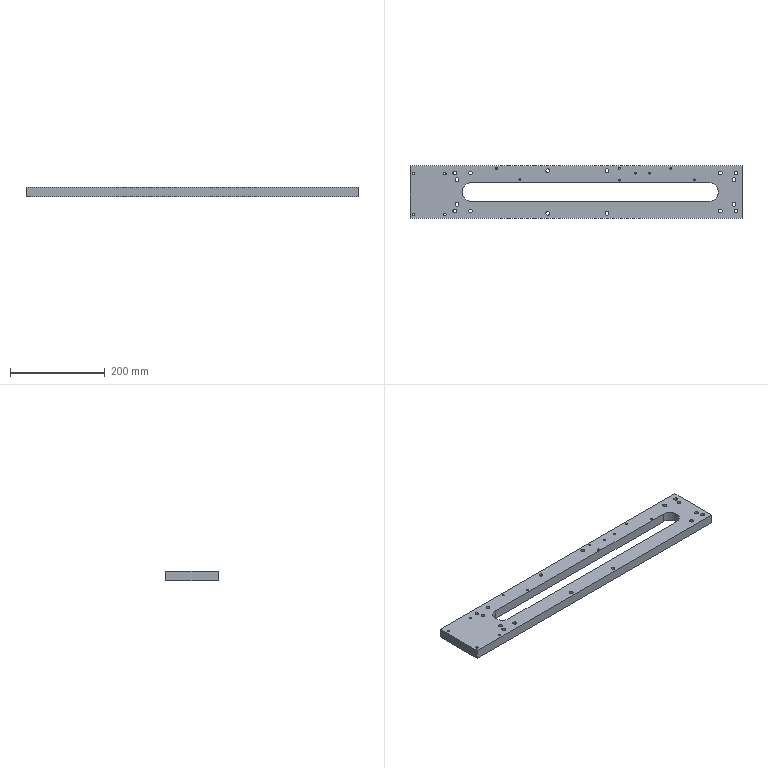Part | STEP file | X77-04001 | 1 solid | 175 faces | box 700 x 110 x 20 mm | volume 1058356 mm3 | cylinder 103 | cone 56 | plane 16 | commonest cylinder face diameters 3.3 x40 8 x32 4.2 x16 5 x8 10 x4 40 x3